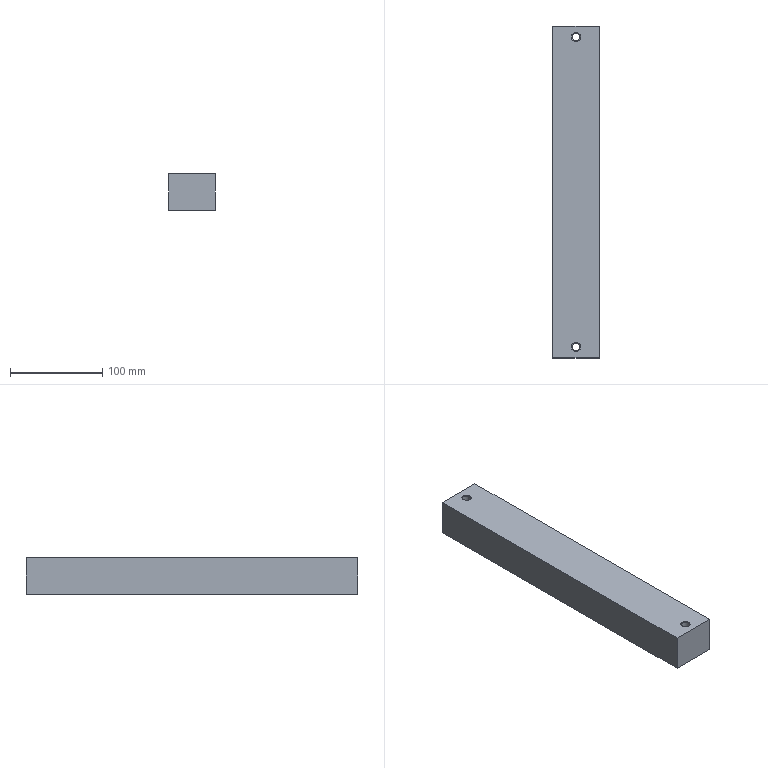Part | STEP file | 1 solid | 12 faces | box 50 x 360 x 40 mm | volume 715429 mm3 | plane 6 | cone 4 | cylinder 2 | commonest cylinder face diameters 8.5 x2
STEP:
#1=CARTESIAN_POINT('',(0.,0.,0.));
#2=DIRECTION('',(0.,0.,1.));
#3=DIRECTION('',(1.,0.,0.));
#4=AXIS2_PLACEMENT_3D('',#1,#2,#3);
#5=CARTESIAN_POINT('',(1866.247,274.48,93.619));
#6=VERTEX_POINT('',#5);
#7=CARTESIAN_POINT('',(1871.247,274.48,93.619));
#8=DIRECTION('',(0.,0.,1.));
#9=DIRECTION('',(-1.,0.,0.));
#10=AXIS2_PLACEMENT_3D('',#7,#8,#9);
#11=CIRCLE('',#10,5.);
#12=CARTESIAN_POINT('',(1846.247,622.48,93.619));
#13=DIRECTION('',(0.,0.,-1.));
#14=DIRECTION('',(0.,1.,0.));
#15=AXIS2_PLACEMENT_3D('',#12,#13,#14);
#16=PLANE('',#15);
#17=CARTESIAN_POINT('',(-348.,20.));
#18=CARTESIAN_POINT('',(-356.66,20.));
#19=CARTESIAN_POINT('',(-352.33,27.5));
#20=CARTESIAN_POINT('',(-348.,35.));
#21=CARTESIAN_POINT('',(-343.67,27.5));
#22=CARTESIAN_POINT('',(-339.34,20.));
#23=CARTESIAN_POINT('',(-348.,20.));
#24=(BOUNDED_CURVE()B_SPLINE_CURVE(2,(#17,#18,#19,#20,#21,#22,#23),.UNSPECIFIED.,.T.,.F.)B_SPLINE_CURVE_WITH_KNOTS((1,2,2,2,2,1),(-2.094,0.,2.094,4.189,6.283,8.378),.UNSPECIFIED.)CURVE()GEOMETRIC_REPRESENTATION_ITEM()RATIONAL_B_SPLINE_CURVE((1.,0.5,1.,0.5,1.,0.5,1.))REPRESENTATION_ITEM(''));
#25=(GEOMETRIC_REPRESENTATION_CONTEXT(2)PARAMETRIC_REPRESENTATION_CONTEXT()REPRESENTATION_CONTEXT('',''));
#26=DEFINITIONAL_REPRESENTATION('',(#24),#25);
#27=PCURVE('',#16,#26);
#28=CARTESIAN_POINT('',(1871.247,274.48,93.619));
#29=DIRECTION('',(0.,0.,-1.));
#30=DIRECTION('',(1.,0.,0.));
#31=AXIS2_PLACEMENT_3D('',#28,#29,#30);
#32=CONICAL_SURFACE('',#31,5.,0.7854);
#33=CARTESIAN_POINT('',(9.425,0.));
#34=DIRECTION('',(-1.,0.));
#35=VECTOR('',#34,1.);
#36=LINE('',#33,#35);
#37=(GEOMETRIC_REPRESENTATION_CONTEXT(2)PARAMETRIC_REPRESENTATION_CONTEXT()REPRESENTATION_CONTEXT('',''));
#38=DEFINITIONAL_REPRESENTATION('',(#36),#37);
#39=PCURVE('',#32,#38);
#40=SURFACE_CURVE('',#11,(#27,#39),.PCURVE_S1.);
#41=EDGE_CURVE('',#6,#6,#40,.T.);
#42=ORIENTED_EDGE('',*,*,#41,.T.);
#43=EDGE_LOOP('',(#42));
#44=FACE_BOUND('',#43,.T.);
#45=CARTESIAN_POINT('',(1866.247,610.48,93.619));
#46=VERTEX_POINT('',#45);
#47=CARTESIAN_POINT('',(1871.247,610.48,93.619));
#48=DIRECTION('',(0.,0.,1.));
#49=DIRECTION('',(-1.,0.,0.));
#50=AXIS2_PLACEMENT_3D('',#47,#48,#49);
#51=CIRCLE('',#50,5.);
#52=CARTESIAN_POINT('',(-12.,20.));
#53=CARTESIAN_POINT('',(-20.66,20.));
#54=CARTESIAN_POINT('',(-16.33,27.5));
#55=CARTESIAN_POINT('',(-12.,35.));
#56=CARTESIAN_POINT('',(-7.67,27.5));
#57=CARTESIAN_POINT('',(-3.34,20.));
#58=CARTESIAN_POINT('',(-12.,20.));
#59=(BOUNDED_CURVE()B_SPLINE_CURVE(2,(#52,#53,#54,#55,#56,#57,#58),.UNSPECIFIED.,.T.,.F.)B_SPLINE_CURVE_WITH_KNOTS((1,2,2,2,2,1),(-2.094,0.,2.094,4.189,6.283,8.378),.UNSPECIFIED.)CURVE()GEOMETRIC_REPRESENTATION_ITEM()RATIONAL_B_SPLINE_CURVE((1.,0.5,1.,0.5,1.,0.5,1.))REPRESENTATION_ITEM(''));
#60=(GEOMETRIC_REPRESENTATION_CONTEXT(2)PARAMETRIC_REPRESENTATION_CONTEXT()REPRESENTATION_CONTEXT('',''));
#61=DEFINITIONAL_REPRESENTATION('',(#59),#60);
#62=PCURVE('',#16,#61);
#63=CARTESIAN_POINT('',(1871.247,610.48,93.619));
#64=DIRECTION('',(0.,0.,-1.));
#65=DIRECTION('',(1.,0.,0.));
#66=AXIS2_PLACEMENT_3D('',#63,#64,#65);
#67=CONICAL_SURFACE('',#66,5.,0.7854);
#68=CARTESIAN_POINT('',(9.425,0.));
#69=DIRECTION('',(-1.,0.));
#70=VECTOR('',#69,1.);
#71=LINE('',#68,#70);
#72=(GEOMETRIC_REPRESENTATION_CONTEXT(2)PARAMETRIC_REPRESENTATION_CONTEXT()REPRESENTATION_CONTEXT('',''));
#73=DEFINITIONAL_REPRESENTATION('',(#71),#72);
#74=PCURVE('',#67,#73);
#75=SURFACE_CURVE('',#51,(#62,#74),.PCURVE_S1.);
#76=EDGE_CURVE('',#46,#46,#75,.T.);
#77=ORIENTED_EDGE('',*,*,#76,.T.);
#78=EDGE_LOOP('',(#77));
#79=FACE_BOUND('',#78,.T.);
#80=CARTESIAN_POINT('',(1846.247,262.48,93.619));
#81=VERTEX_POINT('',#80);
#82=CARTESIAN_POINT('',(1896.247,262.48,93.619));
#83=VERTEX_POINT('',#82);
#84=CARTESIAN_POINT('',(1846.247,262.48,93.619));
#85=DIRECTION('',(1.,0.,0.));
#86=VECTOR('',#85,1.);
#87=LINE('',#84,#86);
#88=CARTESIAN_POINT('',(-360.,0.));
#89=DIRECTION('',(0.,1.));
#90=VECTOR('',#89,1.);
#91=LINE('',#88,#90);
#92=(GEOMETRIC_REPRESENTATION_CONTEXT(2)PARAMETRIC_REPRESENTATION_CONTEXT()REPRESENTATION_CONTEXT('',''));
#93=DEFINITIONAL_REPRESENTATION('',(#91),#92);
#94=PCURVE('',#16,#93);
#95=CARTESIAN_POINT('',(1846.247,262.48,93.619));
#96=DIRECTION('',(0.,-1.,0.));
#97=DIRECTION('',(0.,0.,-1.));
#98=AXIS2_PLACEMENT_3D('',#95,#96,#97);
#99=PLANE('',#98);
#100=CARTESIAN_POINT('',(0.,0.));
#101=DIRECTION('',(0.,1.));
#102=VECTOR('',#101,1.);
#103=LINE('',#100,#102);
#104=(GEOMETRIC_REPRESENTATION_CONTEXT(2)PARAMETRIC_REPRESENTATION_CONTEXT()REPRESENTATION_CONTEXT('',''));
#105=DEFINITIONAL_REPRESENTATION('',(#103),#104);
#106=PCURVE('',#99,#105);
#107=SURFACE_CURVE('',#87,(#94,#106),.PCURVE_S1.);
#108=EDGE_CURVE('',#81,#83,#107,.T.);
#109=ORIENTED_EDGE('',*,*,#108,.F.);
#110=CARTESIAN_POINT('',(1846.247,622.48,93.619));
#111=VERTEX_POINT('',#110);
#112=CARTESIAN_POINT('',(1846.247,622.48,93.619));
#113=DIRECTION('',(0.,-1.,0.));
#114=VECTOR('',#113,1.);
#115=LINE('',#112,#114);
#116=CARTESIAN_POINT('',(0.,0.));
#117=DIRECTION('',(-1.,0.));
#118=VECTOR('',#117,1.);
#119=LINE('',#116,#118);
#120=(GEOMETRIC_REPRESENTATION_CONTEXT(2)PARAMETRIC_REPRESENTATION_CONTEXT()REPRESENTATION_CONTEXT('',''));
#121=DEFINITIONAL_REPRESENTATION('',(#119),#120);
#122=PCURVE('',#16,#121);
#123=CARTESIAN_POINT('',(1846.247,622.48,93.619));
#124=DIRECTION('',(-1.,0.,0.));
#125=DIRECTION('',(0.,1.,0.));
#126=AXIS2_PLACEMENT_3D('',#123,#124,#125);
#127=PLANE('',#126);
#128=CARTESIAN_POINT('',(0.,0.));
#129=DIRECTION('',(-1.,0.));
#130=VECTOR('',#129,1.);
#131=LINE('',#128,#130);
#132=(GEOMETRIC_REPRESENTATION_CONTEXT(2)PARAMETRIC_REPRESENTATION_CONTEXT()REPRESENTATION_CONTEXT('',''));
#133=DEFINITIONAL_REPRESENTATION('',(#131),#132);
#134=PCURVE('',#127,#133);
#135=SURFACE_CURVE('',#115,(#122,#134),.PCURVE_S1.);
#136=EDGE_CURVE('',#111,#81,#135,.T.);
#137=ORIENTED_EDGE('',*,*,#136,.F.);
#138=CARTESIAN_POINT('',(1896.247,622.48,93.619));
#139=VERTEX_POINT('',#138);
#140=CARTESIAN_POINT('',(1846.247,622.48,93.619));
#141=DIRECTION('',(1.,0.,0.));
#142=VECTOR('',#141,1.);
#143=LINE('',#140,#142);
#144=CARTESIAN_POINT('',(0.,0.));
#145=DIRECTION('',(0.,1.));
#146=VECTOR('',#145,1.);
#147=LINE('',#144,#146);
#148=(GEOMETRIC_REPRESENTATION_CONTEXT(2)PARAMETRIC_REPRESENTATION_CONTEXT()REPRESENTATION_CONTEXT('',''));
#149=DEFINITIONAL_REPRESENTATION('',(#147),#148);
#150=PCURVE('',#16,#149);
#151=CARTESIAN_POINT('',(1846.247,622.48,93.619));
#152=DIRECTION('',(0.,-1.,0.));
#153=DIRECTION('',(0.,0.,-1.));
#154=AXIS2_PLACEMENT_3D('',#151,#152,#153);
#155=PLANE('',#154);
#156=CARTESIAN_POINT('',(0.,0.));
#157=DIRECTION('',(0.,1.));
#158=VECTOR('',#157,1.);
#159=LINE('',#156,#158);
#160=(GEOMETRIC_REPRESENTATION_CONTEXT(2)PARAMETRIC_REPRESENTATION_CONTEXT()REPRESENTATION_CONTEXT('',''));
#161=DEFINITIONAL_REPRESENTATION('',(#159),#160);
#162=PCURVE('',#155,#161);
#163=SURFACE_CURVE('',#143,(#150,#162),.PCURVE_S1.);
#164=EDGE_CURVE('',#111,#139,#163,.T.);
#165=ORIENTED_EDGE('',*,*,#164,.T.);
#166=CARTESIAN_POINT('',(1896.247,622.48,93.619));
#167=DIRECTION('',(0.,-1.,0.));
#168=VECTOR('',#167,1.);
#169=LINE('',#166,#168);
#170=CARTESIAN_POINT('',(0.,50.));
#171=DIRECTION('',(-1.,0.));
#172=VECTOR('',#171,1.);
#173=LINE('',#170,#172);
#174=(GEOMETRIC_REPRESENTATION_CONTEXT(2)PARAMETRIC_REPRESENTATION_CONTEXT()REPRESENTATION_CONTEXT('',''));
#175=DEFINITIONAL_REPRESENTATION('',(#173),#174);
#176=PCURVE('',#16,#175);
#177=CARTESIAN_POINT('',(1896.247,622.48,93.619));
#178=DIRECTION('',(-1.,0.,0.));
#179=DIRECTION('',(0.,1.,0.));
#180=AXIS2_PLACEMENT_3D('',#177,#178,#179);
#181=PLANE('',#180);
#182=CARTESIAN_POINT('',(0.,0.));
#183=DIRECTION('',(-1.,0.));
#184=VECTOR('',#183,1.);
#185=LINE('',#182,#184);
#186=(GEOMETRIC_REPRESENTATION_CONTEXT(2)PARAMETRIC_REPRESENTATION_CONTEXT()REPRESENTATION_CONTEXT('',''));
#187=DEFINITIONAL_REPRESENTATION('',(#185),#186);
#188=PCURVE('',#181,#187);
#189=SURFACE_CURVE('',#169,(#176,#188),.PCURVE_S1.);
#190=EDGE_CURVE('',#139,#83,#189,.T.);
#191=ORIENTED_EDGE('',*,*,#190,.T.);
#192=EDGE_LOOP('',(#109,#137,#165,#191));
#193=FACE_BOUND('',#192,.T.);
#194=ADVANCED_FACE('',(#44,#79,#193),#16,.T.);
#195=ORIENTED_EDGE('',*,*,#164,.F.);
#196=CARTESIAN_POINT('',(1846.247,622.48,133.619));
#197=VERTEX_POINT('',#196);
#198=CARTESIAN_POINT('',(1846.247,622.48,93.619));
#199=DIRECTION('',(0.,0.,-1.));
#200=VECTOR('',#199,1.);
#201=LINE('',#198,#200);
#202=CARTESIAN_POINT('',(0.,0.));
#203=DIRECTION('',(1.,0.));
#204=VECTOR('',#203,1.);
#205=LINE('',#202,#204);
#206=(GEOMETRIC_REPRESENTATION_CONTEXT(2)PARAMETRIC_REPRESENTATION_CONTEXT()REPRESENTATION_CONTEXT('',''));
#207=DEFINITIONAL_REPRESENTATION('',(#205),#206);
#208=PCURVE('',#155,#207);
#209=CARTESIAN_POINT('',(0.,0.));
#210=DIRECTION('',(0.,1.));
#211=VECTOR('',#210,1.);
#212=LINE('',#209,#211);
#213=(GEOMETRIC_REPRESENTATION_CONTEXT(2)PARAMETRIC_REPRESENTATION_CONTEXT()REPRESENTATION_CONTEXT('',''));
#214=DEFINITIONAL_REPRESENTATION('',(#212),#213);
#215=PCURVE('',#127,#214);
#216=SURFACE_CURVE('',#201,(#208,#215),.PCURVE_S1.);
#217=EDGE_CURVE('',#197,#111,#216,.T.);
#218=ORIENTED_EDGE('',*,*,#217,.F.);
#219=CARTESIAN_POINT('',(1896.247,622.48,133.619));
#220=VERTEX_POINT('',#219);
#221=CARTESIAN_POINT('',(1846.247,622.48,133.619));
#222=DIRECTION('',(1.,0.,0.));
#223=VECTOR('',#222,1.);
#224=LINE('',#221,#223);
#225=CARTESIAN_POINT('',(-40.,0.));
#226=DIRECTION('',(0.,1.));
#227=VECTOR('',#226,1.);
#228=LINE('',#225,#227);
#229=(GEOMETRIC_REPRESENTATION_CONTEXT(2)PARAMETRIC_REPRESENTATION_CONTEXT()REPRESENTATION_CONTEXT('',''));
#230=DEFINITIONAL_REPRESENTATION('',(#228),#229);
#231=PCURVE('',#155,#230);
#232=CARTESIAN_POINT('',(1846.247,622.48,133.619));
#233=DIRECTION('',(0.,0.,-1.));
#234=DIRECTION('',(0.,1.,0.));
#235=AXIS2_PLACEMENT_3D('',#232,#233,#234);
#236=PLANE('',#235);
#237=CARTESIAN_POINT('',(0.,0.));
#238=DIRECTION('',(0.,1.));
#239=VECTOR('',#238,1.);
#240=LINE('',#237,#239);
#241=(GEOMETRIC_REPRESENTATION_CONTEXT(2)PARAMETRIC_REPRESENTATION_CONTEXT()REPRESENTATION_CONTEXT('',''));
#242=DEFINITIONAL_REPRESENTATION('',(#240),#241);
#243=PCURVE('',#236,#242);
#244=SURFACE_CURVE('',#224,(#231,#243),.PCURVE_S1.);
#245=EDGE_CURVE('',#197,#220,#244,.T.);
#246=ORIENTED_EDGE('',*,*,#245,.T.);
#247=CARTESIAN_POINT('',(1896.247,622.48,93.619));
#248=DIRECTION('',(0.,0.,-1.));
#249=VECTOR('',#248,1.);
#250=LINE('',#247,#249);
#251=CARTESIAN_POINT('',(0.,50.));
#252=DIRECTION('',(1.,0.));
#253=VECTOR('',#252,1.);
#254=LINE('',#251,#253);
#255=(GEOMETRIC_REPRESENTATION_CONTEXT(2)PARAMETRIC_REPRESENTATION_CONTEXT()REPRESENTATION_CONTEXT('',''));
#256=DEFINITIONAL_REPRESENTATION('',(#254),#255);
#257=PCURVE('',#155,#256);
#258=CARTESIAN_POINT('',(0.,0.));
#259=DIRECTION('',(0.,1.));
#260=VECTOR('',#259,1.);
#261=LINE('',#258,#260);
#262=(GEOMETRIC_REPRESENTATION_CONTEXT(2)PARAMETRIC_REPRESENTATION_CONTEXT()REPRESENTATION_CONTEXT('',''));
#263=DEFINITIONAL_REPRESENTATION('',(#261),#262);
#264=PCURVE('',#181,#263);
#265=SURFACE_CURVE('',#250,(#257,#264),.PCURVE_S1.);
#266=EDGE_CURVE('',#220,#139,#265,.T.);
#267=ORIENTED_EDGE('',*,*,#266,.T.);
#268=EDGE_LOOP('',(#195,#218,#246,#267));
#269=FACE_BOUND('',#268,.T.);
#270=ADVANCED_FACE('',(#269),#155,.F.);
#271=CARTESIAN_POINT('',(1866.247,274.48,133.619));
#272=VERTEX_POINT('',#271);
#273=CARTESIAN_POINT('',(1871.247,274.48,133.619));
#274=DIRECTION('',(0.,0.,-1.));
#275=DIRECTION('',(-1.,0.,0.));
#276=AXIS2_PLACEMENT_3D('',#273,#274,#275);
#277=CIRCLE('',#276,5.);
#278=CARTESIAN_POINT('',(-348.,25.));
#279=DIRECTION('',(0.,-1.));
#280=AXIS2_PLACEMENT_2D('',#278,#279);
#281=CIRCLE('',#280,5.);
#282=(GEOMETRIC_REPRESENTATION_CONTEXT(2)PARAMETRIC_REPRESENTATION_CONTEXT()REPRESENTATION_CONTEXT('',''));
#283=DEFINITIONAL_REPRESENTATION('',(#281),#282);
#284=PCURVE('',#236,#283);
#285=CARTESIAN_POINT('',(1871.247,274.48,132.869));
#286=DIRECTION('',(0.,0.,1.));
#287=DIRECTION('',(-1.,0.,0.));
#288=AXIS2_PLACEMENT_3D('',#285,#286,#287);
#289=CONICAL_SURFACE('',#288,4.25,0.7854);
#290=CARTESIAN_POINT('',(6.283,0.75));
#291=DIRECTION('',(-1.,0.));
#292=VECTOR('',#291,1.);
#293=LINE('',#290,#292);
#294=(GEOMETRIC_REPRESENTATION_CONTEXT(2)PARAMETRIC_REPRESENTATION_CONTEXT()REPRESENTATION_CONTEXT('',''));
#295=DEFINITIONAL_REPRESENTATION('',(#293),#294);
#296=PCURVE('',#289,#295);
#297=SURFACE_CURVE('',#277,(#284,#296),.PCURVE_S1.);
#298=EDGE_CURVE('',#272,#272,#297,.T.);
#299=ORIENTED_EDGE('',*,*,#298,.T.);
#300=EDGE_LOOP('',(#299));
#301=FACE_BOUND('',#300,.T.);
#302=CARTESIAN_POINT('',(1866.247,610.48,133.619));
#303=VERTEX_POINT('',#302);
#304=CARTESIAN_POINT('',(1871.247,610.48,133.619));
#305=DIRECTION('',(0.,0.,-1.));
#306=DIRECTION('',(-1.,0.,0.));
#307=AXIS2_PLACEMENT_3D('',#304,#305,#306);
#308=CIRCLE('',#307,5.);
#309=CARTESIAN_POINT('',(-12.,25.));
#310=DIRECTION('',(0.,-1.));
#311=AXIS2_PLACEMENT_2D('',#309,#310);
#312=CIRCLE('',#311,5.);
#313=(GEOMETRIC_REPRESENTATION_CONTEXT(2)PARAMETRIC_REPRESENTATION_CONTEXT()REPRESENTATION_CONTEXT('',''));
#314=DEFINITIONAL_REPRESENTATION('',(#312),#313);
#315=PCURVE('',#236,#314);
#316=CARTESIAN_POINT('',(1871.247,610.48,132.869));
#317=DIRECTION('',(0.,0.,1.));
#318=DIRECTION('',(-1.,0.,0.));
#319=AXIS2_PLACEMENT_3D('',#316,#317,#318);
#320=CONICAL_SURFACE('',#319,4.25,0.7854);
#321=CARTESIAN_POINT('',(6.283,0.75));
#322=DIRECTION('',(-1.,0.));
#323=VECTOR('',#322,1.);
#324=LINE('',#321,#323);
#325=(GEOMETRIC_REPRESENTATION_CONTEXT(2)PARAMETRIC_REPRESENTATION_CONTEXT()REPRESENTATION_CONTEXT('',''));
#326=DEFINITIONAL_REPRESENTATION('',(#324),#325);
#327=PCURVE('',#320,#326);
#328=SURFACE_CURVE('',#308,(#315,#327),.PCURVE_S1.);
#329=EDGE_CURVE('',#303,#303,#328,.T.);
#330=ORIENTED_EDGE('',*,*,#329,.T.);
#331=EDGE_LOOP('',(#330));
#332=FACE_BOUND('',#331,.T.);
#333=ORIENTED_EDGE('',*,*,#245,.F.);
#334=CARTESIAN_POINT('',(1846.247,262.48,133.619));
#335=VERTEX_POINT('',#334);
#336=CARTESIAN_POINT('',(1846.247,622.48,133.619));
#337=DIRECTION('',(0.,1.,0.));
#338=VECTOR('',#337,1.);
#339=LINE('',#336,#338);
#340=CARTESIAN_POINT('',(0.,0.));
#341=DIRECTION('',(1.,0.));
#342=VECTOR('',#341,1.);
#343=LINE('',#340,#342);
#344=(GEOMETRIC_REPRESENTATION_CONTEXT(2)PARAMETRIC_REPRESENTATION_CONTEXT()REPRESENTATION_CONTEXT('',''));
#345=DEFINITIONAL_REPRESENTATION('',(#343),#344);
#346=PCURVE('',#236,#345);
#347=CARTESIAN_POINT('',(0.,-40.));
#348=DIRECTION('',(1.,0.));
#349=VECTOR('',#348,1.);
#350=LINE('',#347,#349);
#351=(GEOMETRIC_REPRESENTATION_CONTEXT(2)PARAMETRIC_REPRESENTATION_CONTEXT()REPRESENTATION_CONTEXT('',''));
#352=DEFINITIONAL_REPRESENTATION('',(#350),#351);
#353=PCURVE('',#127,#352);
#354=SURFACE_CURVE('',#339,(#346,#353),.PCURVE_S1.);
#355=EDGE_CURVE('',#335,#197,#354,.T.);
#356=ORIENTED_EDGE('',*,*,#355,.F.);
#357=CARTESIAN_POINT('',(1896.247,262.48,133.619));
#358=VERTEX_POINT('',#357);
#359=CARTESIAN_POINT('',(1846.247,262.48,133.619));
#360=DIRECTION('',(1.,0.,0.));
#361=VECTOR('',#360,1.);
#362=LINE('',#359,#361);
#363=CARTESIAN_POINT('',(-360.,0.));
#364=DIRECTION('',(0.,1.));
#365=VECTOR('',#364,1.);
#366=LINE('',#363,#365);
#367=(GEOMETRIC_REPRESENTATION_CONTEXT(2)PARAMETRIC_REPRESENTATION_CONTEXT()REPRESENTATION_CONTEXT('',''));
#368=DEFINITIONAL_REPRESENTATION('',(#366),#367);
#369=PCURVE('',#236,#368);
#370=CARTESIAN_POINT('',(-40.,0.));
#371=DIRECTION('',(0.,1.));
#372=VECTOR('',#371,1.);
#373=LINE('',#370,#372);
#374=(GEOMETRIC_REPRESENTATION_CONTEXT(2)PARAMETRIC_REPRESENTATION_CONTEXT()REPRESENTATION_CONTEXT('',''));
#375=DEFINITIONAL_REPRESENTATION('',(#373),#374);
#376=PCURVE('',#99,#375);
#377=SURFACE_CURVE('',#362,(#369,#376),.PCURVE_S1.);
#378=EDGE_CURVE('',#335,#358,#377,.T.);
#379=ORIENTED_EDGE('',*,*,#378,.T.);
#380=CARTESIAN_POINT('',(1896.247,622.48,133.619));
#381=DIRECTION('',(0.,1.,0.));
#382=VECTOR('',#381,1.);
#383=LINE('',#380,#382);
#384=CARTESIAN_POINT('',(0.,50.));
#385=DIRECTION('',(1.,0.));
#386=VECTOR('',#385,1.);
#387=LINE('',#384,#386);
#388=(GEOMETRIC_REPRESENTATION_CONTEXT(2)PARAMETRIC_REPRESENTATION_CONTEXT()REPRESENTATION_CONTEXT('',''));
#389=DEFINITIONAL_REPRESENTATION('',(#387),#388);
#390=PCURVE('',#236,#389);
#391=CARTESIAN_POINT('',(0.,-40.));
#392=DIRECTION('',(1.,0.));
#393=VECTOR('',#392,1.);
#394=LINE('',#391,#393);
#395=(GEOMETRIC_REPRESENTATION_CONTEXT(2)PARAMETRIC_REPRESENTATION_CONTEXT()REPRESENTATION_CONTEXT('',''));
#396=DEFINITIONAL_REPRESENTATION('',(#394),#395);
#397=PCURVE('',#181,#396);
#398=SURFACE_CURVE('',#383,(#390,#397),.PCURVE_S1.);
#399=EDGE_CURVE('',#358,#220,#398,.T.);
#400=ORIENTED_EDGE('',*,*,#399,.T.);
#401=EDGE_LOOP('',(#333,#356,#379,#400));
#402=FACE_BOUND('',#401,.T.);
#403=ADVANCED_FACE('',(#301,#332,#402),#236,.F.);
#404=CARTESIAN_POINT('',(1846.247,262.48,93.619));
#405=DIRECTION('',(0.,0.,1.));
#406=VECTOR('',#405,1.);
#407=LINE('',#404,#406);
#408=CARTESIAN_POINT('',(0.,0.));
#409=DIRECTION('',(-1.,0.));
#410=VECTOR('',#409,1.);
#411=LINE('',#408,#410);
#412=(GEOMETRIC_REPRESENTATION_CONTEXT(2)PARAMETRIC_REPRESENTATION_CONTEXT()REPRESENTATION_CONTEXT('',''));
#413=DEFINITIONAL_REPRESENTATION('',(#411),#412);
#414=PCURVE('',#99,#413);
#415=CARTESIAN_POINT('',(-360.,0.));
#416=DIRECTION('',(0.,-1.));
#417=VECTOR('',#416,1.);
#418=LINE('',#415,#417);
#419=(GEOMETRIC_REPRESENTATION_CONTEXT(2)PARAMETRIC_REPRESENTATION_CONTEXT()REPRESENTATION_CONTEXT('',''));
#420=DEFINITIONAL_REPRESENTATION('',(#418),#419);
#421=PCURVE('',#127,#420);
#422=SURFACE_CURVE('',#407,(#414,#421),.PCURVE_S1.);
#423=EDGE_CURVE('',#81,#335,#422,.T.);
#424=ORIENTED_EDGE('',*,*,#423,.F.);
#425=ORIENTED_EDGE('',*,*,#108,.T.);
#426=CARTESIAN_POINT('',(1896.247,262.48,93.619));
#427=DIRECTION('',(0.,0.,1.));
#428=VECTOR('',#427,1.);
#429=LINE('',#426,#428);
#430=CARTESIAN_POINT('',(0.,50.));
#431=DIRECTION('',(-1.,0.));
#432=VECTOR('',#431,1.);
#433=LINE('',#430,#432);
#434=(GEOMETRIC_REPRESENTATION_CONTEXT(2)PARAMETRIC_REPRESENTATION_CONTEXT()REPRESENTATION_CONTEXT('',''));
#435=DEFINITIONAL_REPRESENTATION('',(#433),#434);
#436=PCURVE('',#99,#435);
#437=CARTESIAN_POINT('',(-360.,0.));
#438=DIRECTION('',(0.,-1.));
#439=VECTOR('',#438,1.);
#440=LINE('',#437,#439);
#441=(GEOMETRIC_REPRESENTATION_CONTEXT(2)PARAMETRIC_REPRESENTATION_CONTEXT()REPRESENTATION_CONTEXT('',''));
#442=DEFINITIONAL_REPRESENTATION('',(#440),#441);
#443=PCURVE('',#181,#442);
#444=SURFACE_CURVE('',#429,(#436,#443),.PCURVE_S1.);
#445=EDGE_CURVE('',#83,#358,#444,.T.);
#446=ORIENTED_EDGE('',*,*,#445,.T.);
#447=ORIENTED_EDGE('',*,*,#378,.F.);
#448=EDGE_LOOP('',(#424,#425,#446,#447));
#449=FACE_BOUND('',#448,.T.);
#450=ADVANCED_FACE('',(#449),#99,.T.);
#451=ORIENTED_EDGE('',*,*,#399,.F.);
#452=ORIENTED_EDGE('',*,*,#445,.F.);
#453=ORIENTED_EDGE('',*,*,#190,.F.);
#454=ORIENTED_EDGE('',*,*,#266,.F.);
#455=EDGE_LOOP('',(#451,#452,#453,#454));
#456=FACE_BOUND('',#455,.T.);
#457=ADVANCED_FACE('',(#456),#181,.F.);
#458=ORIENTED_EDGE('',*,*,#355,.T.);
#459=ORIENTED_EDGE('',*,*,#217,.T.);
#460=ORIENTED_EDGE('',*,*,#136,.T.);
#461=ORIENTED_EDGE('',*,*,#423,.T.);
#462=EDGE_LOOP('',(#458,#459,#460,#461));
#463=FACE_BOUND('',#462,.T.);
#464=ADVANCED_FACE('',(#463),#127,.T.);
#465=CARTESIAN_POINT('',(1866.997,610.48,132.869));
#466=VERTEX_POINT('',#465);
#467=CARTESIAN_POINT('',(1875.497,610.48,132.869));
#468=VERTEX_POINT('',#467);
#469=CARTESIAN_POINT('',(1871.247,610.48,132.869));
#470=DIRECTION('',(0.,0.,1.));
#471=DIRECTION('',(1.,0.,0.));
#472=AXIS2_PLACEMENT_3D('',#469,#470,#471);
#473=CIRCLE('',#472,4.25);
#474=CARTESIAN_POINT('',(1871.247,610.48,93.619));
#475=DIRECTION('',(0.,0.,1.));
#476=DIRECTION('',(-1.,0.,0.));
#477=AXIS2_PLACEMENT_3D('',#474,#475,#476);
#478=CYLINDRICAL_SURFACE('',#477,4.25);
#479=CARTESIAN_POINT('',(-3.142,39.25));
#480=DIRECTION('',(1.,0.));
#481=VECTOR('',#480,1.);
#482=LINE('',#479,#481);
#483=(GEOMETRIC_REPRESENTATION_CONTEXT(2)PARAMETRIC_REPRESENTATION_CONTEXT()REPRESENTATION_CONTEXT('',''));
#484=DEFINITIONAL_REPRESENTATION('',(#482),#483);
#485=PCURVE('',#478,#484);
#486=CARTESIAN_POINT('',(-3.142,0.));
#487=DIRECTION('',(1.,0.));
#488=VECTOR('',#487,1.);
#489=LINE('',#486,#488);
#490=(GEOMETRIC_REPRESENTATION_CONTEXT(2)PARAMETRIC_REPRESENTATION_CONTEXT()REPRESENTATION_CONTEXT('',''));
#491=DEFINITIONAL_REPRESENTATION('',(#489),#490);
#492=PCURVE('',#320,#491);
#493=SURFACE_CURVE('',#473,(#485,#492),.PCURVE_S1.);
#494=EDGE_CURVE('',#466,#468,#493,.T.);
#495=ORIENTED_EDGE('',*,*,#494,.F.);
#496=CARTESIAN_POINT('',(1866.997,610.48,94.369));
#497=VERTEX_POINT('',#496);
#498=CARTESIAN_POINT('',(1866.997,610.48,94.369));
#499=CARTESIAN_POINT('',(1866.997,610.48,132.869));
#500=B_SPLINE_CURVE_WITH_KNOTS('',1,(#498,#499),.UNSPECIFIED.,.F.,.F.,(2,2),(0.75,39.25),.PIECEWISE_BEZIER_KNOTS.);
#501=CARTESIAN_POINT('',(0.,0.));
#502=DIRECTION('',(0.,1.));
#503=VECTOR('',#502,1.);
#504=LINE('',#501,#503);
#505=(GEOMETRIC_REPRESENTATION_CONTEXT(2)PARAMETRIC_REPRESENTATION_CONTEXT()REPRESENTATION_CONTEXT('',''));
#506=DEFINITIONAL_REPRESENTATION('',(#504),#505);
#507=PCURVE('',#478,#506);
#508=CARTESIAN_POINT('',(6.283,0.));
#509=DIRECTION('',(0.,1.));
#510=VECTOR('',#509,1.);
#511=LINE('',#508,#510);
#512=(GEOMETRIC_REPRESENTATION_CONTEXT(2)PARAMETRIC_REPRESENTATION_CONTEXT()REPRESENTATION_CONTEXT('',''));
#513=DEFINITIONAL_REPRESENTATION('',(#511),#512);
#514=PCURVE('',#478,#513);
#515=SEAM_CURVE('',#500,(#507,#514),.PCURVE_S1.);
#516=EDGE_CURVE('',#497,#466,#515,.T.);
#517=ORIENTED_EDGE('',*,*,#516,.F.);
#518=CARTESIAN_POINT('',(1871.247,610.48,94.369));
#519=DIRECTION('',(0.,0.,-1.));
#520=DIRECTION('',(-1.,0.,0.));
#521=AXIS2_PLACEMENT_3D('',#518,#519,#520);
#522=CIRCLE('',#521,4.25);
#523=CARTESIAN_POINT('',(6.283,0.75));
#524=DIRECTION('',(-1.,0.));
#525=VECTOR('',#524,1.);
#526=LINE('',#523,#525);
#527=(GEOMETRIC_REPRESENTATION_CONTEXT(2)PARAMETRIC_REPRESENTATION_CONTEXT()REPRESENTATION_CONTEXT('',''));
#528=DEFINITIONAL_REPRESENTATION('',(#526),#527);
#529=PCURVE('',#478,#528);
#530=CARTESIAN_POINT('',(3.142,-0.75));
#531=DIRECTION('',(1.,0.));
#532=VECTOR('',#531,1.);
#533=LINE('',#530,#532);
#534=(GEOMETRIC_REPRESENTATION_CONTEXT(2)PARAMETRIC_REPRESENTATION_CONTEXT()REPRESENTATION_CONTEXT('',''));
#535=DEFINITIONAL_REPRESENTATION('',(#533),#534);
#536=PCURVE('',#67,#535);
#537=SURFACE_CURVE('',#522,(#529,#536),.PCURVE_S1.);
#538=EDGE_CURVE('',#497,#497,#537,.T.);
#539=ORIENTED_EDGE('',*,*,#538,.F.);
#540=ORIENTED_EDGE('',*,*,#516,.T.);
#541=CARTESIAN_POINT('',(1871.247,610.48,132.869));
#542=DIRECTION('',(0.,0.,1.));
#543=DIRECTION('',(1.,0.,0.));
#544=AXIS2_PLACEMENT_3D('',#541,#542,#543);
#545=CIRCLE('',#544,4.25);
#546=CARTESIAN_POINT('',(3.142,39.25));
#547=DIRECTION('',(1.,0.));
#548=VECTOR('',#547,1.);
#549=LINE('',#546,#548);
#550=(GEOMETRIC_REPRESENTATION_CONTEXT(2)PARAMETRIC_REPRESENTATION_CONTEXT()REPRESENTATION_CONTEXT('',''));
#551=DEFINITIONAL_REPRESENTATION('',(#549),#550);
#552=PCURVE('',#478,#551);
#553=CARTESIAN_POINT('',(3.142,0.));
#554=DIRECTION('',(1.,0.));
#555=VECTOR('',#554,1.);
#556=LINE('',#553,#555);
#557=(GEOMETRIC_REPRESENTATION_CONTEXT(2)PARAMETRIC_REPRESENTATION_CONTEXT()REPRESENTATION_CONTEXT('',''));
#558=DEFINITIONAL_REPRESENTATION('',(#556),#557);
#559=PCURVE('',#320,#558);
#560=SURFACE_CURVE('',#545,(#552,#559),.PCURVE_S1.);
#561=EDGE_CURVE('',#468,#466,#560,.T.);
#562=ORIENTED_EDGE('',*,*,#561,.F.);
#563=EDGE_LOOP('',(#495,#517,#539,#540,#562));
#564=FACE_BOUND('',#563,.F.);
#565=ADVANCED_FACE('',(#564),#478,.F.);
#566=ORIENTED_EDGE('',*,*,#538,.T.);
#567=CARTESIAN_POINT('',(1866.997,610.48,94.369));
#568=CARTESIAN_POINT('',(1866.247,610.48,93.619));
#569=B_SPLINE_CURVE_WITH_KNOTS('',1,(#567,#568),.UNSPECIFIED.,.F.,.F.,(2,2),(-1.061,0.),.PIECEWISE_BEZIER_KNOTS.);
#570=CARTESIAN_POINT('',(9.425,0.));
#571=DIRECTION('',(0.,1.));
#572=VECTOR('',#571,1.);
#573=LINE('',#570,#572);
#574=(GEOMETRIC_REPRESENTATION_CONTEXT(2)PARAMETRIC_REPRESENTATION_CONTEXT()REPRESENTATION_CONTEXT('',''));
#575=DEFINITIONAL_REPRESENTATION('',(#573),#574);
#576=PCURVE('',#67,#575);
#577=CARTESIAN_POINT('',(3.142,0.));
#578=DIRECTION('',(0.,1.));
#579=VECTOR('',#578,1.);
#580=LINE('',#577,#579);
#581=(GEOMETRIC_REPRESENTATION_CONTEXT(2)PARAMETRIC_REPRESENTATION_CONTEXT()REPRESENTATION_CONTEXT('',''));
#582=DEFINITIONAL_REPRESENTATION('',(#580),#581);
#583=PCURVE('',#67,#582);
#584=SEAM_CURVE('',#569,(#576,#583),.PCURVE_S1.);
#585=EDGE_CURVE('',#497,#46,#584,.T.);
#586=ORIENTED_EDGE('',*,*,#585,.T.);
#587=ORIENTED_EDGE('',*,*,#76,.T.);
#588=ORIENTED_EDGE('',*,*,#585,.F.);
#589=EDGE_LOOP('',(#566,#586,#587,#588));
#590=FACE_BOUND('',#589,.F.);
#591=ADVANCED_FACE('',(#590),#67,.F.);
#592=ORIENTED_EDGE('',*,*,#329,.T.);
#593=CARTESIAN_POINT('',(1866.997,610.48,132.869));
#594=CARTESIAN_POINT('',(1866.247,610.48,133.619));
#595=B_SPLINE_CURVE_WITH_KNOTS('',1,(#593,#594),.UNSPECIFIED.,.F.,.F.,(2,2),(0.,1.061),.PIECEWISE_BEZIER_KNOTS.);
#596=CARTESIAN_POINT('',(0.,0.));
#597=DIRECTION('',(0.,1.));
#598=VECTOR('',#597,1.);
#599=LINE('',#596,#598);
#600=(GEOMETRIC_REPRESENTATION_CONTEXT(2)PARAMETRIC_REPRESENTATION_CONTEXT()REPRESENTATION_CONTEXT('',''));
#601=DEFINITIONAL_REPRESENTATION('',(#599),#600);
#602=PCURVE('',#320,#601);
#603=CARTESIAN_POINT('',(6.283,0.));
#604=DIRECTION('',(0.,1.));
#605=VECTOR('',#604,1.);
#606=LINE('',#603,#605);
#607=(GEOMETRIC_REPRESENTATION_CONTEXT(2)PARAMETRIC_REPRESENTATION_CONTEXT()REPRESENTATION_CONTEXT('',''));
#608=DEFINITIONAL_REPRESENTATION('',(#606),#607);
#609=PCURVE('',#320,#608);
#610=SEAM_CURVE('',#595,(#602,#609),.PCURVE_S1.);
#611=EDGE_CURVE('',#466,#303,#610,.T.);
#612=ORIENTED_EDGE('',*,*,#611,.F.);
#613=ORIENTED_EDGE('',*,*,#494,.T.);
#614=ORIENTED_EDGE('',*,*,#561,.T.);
#615=ORIENTED_EDGE('',*,*,#611,.T.);
#616=EDGE_LOOP('',(#592,#612,#613,#614,#615));
#617=FACE_BOUND('',#616,.F.);
#618=ADVANCED_FACE('',(#617),#320,.F.);
#619=CARTESIAN_POINT('',(1866.997,274.48,132.869));
#620=VERTEX_POINT('',#619);
#621=CARTESIAN_POINT('',(1875.497,274.48,132.869));
#622=VERTEX_POINT('',#621);
#623=CARTESIAN_POINT('',(1871.247,274.48,132.869));
#624=DIRECTION('',(0.,0.,1.));
#625=DIRECTION('',(1.,0.,0.));
#626=AXIS2_PLACEMENT_3D('',#623,#624,#625);
#627=CIRCLE('',#626,4.25);
#628=CARTESIAN_POINT('',(1871.247,274.48,93.619));
#629=DIRECTION('',(0.,0.,1.));
#630=DIRECTION('',(-1.,0.,0.));
#631=AXIS2_PLACEMENT_3D('',#628,#629,#630);
#632=CYLINDRICAL_SURFACE('',#631,4.25);
#633=CARTESIAN_POINT('',(-3.142,39.25));
#634=DIRECTION('',(1.,0.));
#635=VECTOR('',#634,1.);
#636=LINE('',#633,#635);
#637=(GEOMETRIC_REPRESENTATION_CONTEXT(2)PARAMETRIC_REPRESENTATION_CONTEXT()REPRESENTATION_CONTEXT('',''));
#638=DEFINITIONAL_REPRESENTATION('',(#636),#637);
#639=PCURVE('',#632,#638);
#640=CARTESIAN_POINT('',(-3.142,0.));
#641=DIRECTION('',(1.,0.));
#642=VECTOR('',#641,1.);
#643=LINE('',#640,#642);
#644=(GEOMETRIC_REPRESENTATION_CONTEXT(2)PARAMETRIC_REPRESENTATION_CONTEXT()REPRESENTATION_CONTEXT('',''));
#645=DEFINITIONAL_REPRESENTATION('',(#643),#644);
#646=PCURVE('',#289,#645);
#647=SURFACE_CURVE('',#627,(#639,#646),.PCURVE_S1.);
#648=EDGE_CURVE('',#620,#622,#647,.T.);
#649=ORIENTED_EDGE('',*,*,#648,.F.);
#650=CARTESIAN_POINT('',(1866.997,274.48,94.369));
#651=VERTEX_POINT('',#650);
#652=CARTESIAN_POINT('',(1866.997,274.48,94.369));
#653=CARTESIAN_POINT('',(1866.997,274.48,132.869));
#654=B_SPLINE_CURVE_WITH_KNOTS('',1,(#652,#653),.UNSPECIFIED.,.F.,.F.,(2,2),(0.75,39.25),.PIECEWISE_BEZIER_KNOTS.);
#655=CARTESIAN_POINT('',(0.,0.));
#656=DIRECTION('',(0.,1.));
#657=VECTOR('',#656,1.);
#658=LINE('',#655,#657);
#659=(GEOMETRIC_REPRESENTATION_CONTEXT(2)PARAMETRIC_REPRESENTATION_CONTEXT()REPRESENTATION_CONTEXT('',''));
#660=DEFINITIONAL_REPRESENTATION('',(#658),#659);
#661=PCURVE('',#632,#660);
#662=CARTESIAN_POINT('',(6.283,0.));
#663=DIRECTION('',(0.,1.));
#664=VECTOR('',#663,1.);
#665=LINE('',#662,#664);
#666=(GEOMETRIC_REPRESENTATION_CONTEXT(2)PARAMETRIC_REPRESENTATION_CONTEXT()REPRESENTATION_CONTEXT('',''));
#667=DEFINITIONAL_REPRESENTATION('',(#665),#666);
#668=PCURVE('',#632,#667);
#669=SEAM_CURVE('',#654,(#661,#668),.PCURVE_S1.);
#670=EDGE_CURVE('',#651,#620,#669,.T.);
#671=ORIENTED_EDGE('',*,*,#670,.F.);
#672=CARTESIAN_POINT('',(1871.247,274.48,94.369));
#673=DIRECTION('',(0.,0.,-1.));
#674=DIRECTION('',(-1.,0.,0.));
#675=AXIS2_PLACEMENT_3D('',#672,#673,#674);
#676=CIRCLE('',#675,4.25);
#677=CARTESIAN_POINT('',(6.283,0.75));
#678=DIRECTION('',(-1.,0.));
#679=VECTOR('',#678,1.);
#680=LINE('',#677,#679);
#681=(GEOMETRIC_REPRESENTATION_CONTEXT(2)PARAMETRIC_REPRESENTATION_CONTEXT()REPRESENTATION_CONTEXT('',''));
#682=DEFINITIONAL_REPRESENTATION('',(#680),#681);
#683=PCURVE('',#632,#682);
#684=CARTESIAN_POINT('',(3.142,-0.75));
#685=DIRECTION('',(1.,0.));
#686=VECTOR('',#685,1.);
#687=LINE('',#684,#686);
#688=(GEOMETRIC_REPRESENTATION_CONTEXT(2)PARAMETRIC_REPRESENTATION_CONTEXT()REPRESENTATION_CONTEXT('',''));
#689=DEFINITIONAL_REPRESENTATION('',(#687),#688);
#690=PCURVE('',#32,#689);
#691=SURFACE_CURVE('',#676,(#683,#690),.PCURVE_S1.);
#692=EDGE_CURVE('',#651,#651,#691,.T.);
#693=ORIENTED_EDGE('',*,*,#692,.F.);
#694=ORIENTED_EDGE('',*,*,#670,.T.);
#695=CARTESIAN_POINT('',(1871.247,274.48,132.869));
#696=DIRECTION('',(0.,0.,1.));
#697=DIRECTION('',(1.,0.,0.));
#698=AXIS2_PLACEMENT_3D('',#695,#696,#697);
#699=CIRCLE('',#698,4.25);
#700=CARTESIAN_POINT('',(3.142,39.25));
#701=DIRECTION('',(1.,0.));
#702=VECTOR('',#701,1.);
#703=LINE('',#700,#702);
#704=(GEOMETRIC_REPRESENTATION_CONTEXT(2)PARAMETRIC_REPRESENTATION_CONTEXT()REPRESENTATION_CONTEXT('',''));
#705=DEFINITIONAL_REPRESENTATION('',(#703),#704);
#706=PCURVE('',#632,#705);
#707=CARTESIAN_POINT('',(3.142,0.));
#708=DIRECTION('',(1.,0.));
#709=VECTOR('',#708,1.);
#710=LINE('',#707,#709);
#711=(GEOMETRIC_REPRESENTATION_CONTEXT(2)PARAMETRIC_REPRESENTATION_CONTEXT()REPRESENTATION_CONTEXT('',''));
#712=DEFINITIONAL_REPRESENTATION('',(#710),#711);
#713=PCURVE('',#289,#712);
#714=SURFACE_CURVE('',#699,(#706,#713),.PCURVE_S1.);
#715=EDGE_CURVE('',#622,#620,#714,.T.);
#716=ORIENTED_EDGE('',*,*,#715,.F.);
#717=EDGE_LOOP('',(#649,#671,#693,#694,#716));
#718=FACE_BOUND('',#717,.F.);
#719=ADVANCED_FACE('',(#718),#632,.F.);
#720=ORIENTED_EDGE('',*,*,#692,.T.);
#721=CARTESIAN_POINT('',(1866.997,274.48,94.369));
#722=CARTESIAN_POINT('',(1866.247,274.48,93.619));
#723=B_SPLINE_CURVE_WITH_KNOTS('',1,(#721,#722),.UNSPECIFIED.,.F.,.F.,(2,2),(-1.061,0.),.PIECEWISE_BEZIER_KNOTS.);
#724=CARTESIAN_POINT('',(9.425,0.));
#725=DIRECTION('',(0.,1.));
#726=VECTOR('',#725,1.);
#727=LINE('',#724,#726);
#728=(GEOMETRIC_REPRESENTATION_CONTEXT(2)PARAMETRIC_REPRESENTATION_CONTEXT()REPRESENTATION_CONTEXT('',''));
#729=DEFINITIONAL_REPRESENTATION('',(#727),#728);
#730=PCURVE('',#32,#729);
#731=CARTESIAN_POINT('',(3.142,0.));
#732=DIRECTION('',(0.,1.));
#733=VECTOR('',#732,1.);
#734=LINE('',#731,#733);
#735=(GEOMETRIC_REPRESENTATION_CONTEXT(2)PARAMETRIC_REPRESENTATION_CONTEXT()REPRESENTATION_CONTEXT('',''));
#736=DEFINITIONAL_REPRESENTATION('',(#734),#735);
#737=PCURVE('',#32,#736);
#738=SEAM_CURVE('',#723,(#730,#737),.PCURVE_S1.);
#739=EDGE_CURVE('',#651,#6,#738,.T.);
#740=ORIENTED_EDGE('',*,*,#739,.T.);
#741=ORIENTED_EDGE('',*,*,#41,.T.);
#742=ORIENTED_EDGE('',*,*,#739,.F.);
#743=EDGE_LOOP('',(#720,#740,#741,#742));
#744=FACE_BOUND('',#743,.F.);
#745=ADVANCED_FACE('',(#744),#32,.F.);
#746=ORIENTED_EDGE('',*,*,#298,.T.);
#747=CARTESIAN_POINT('',(1866.997,274.48,132.869));
#748=CARTESIAN_POINT('',(1866.247,274.48,133.619));
#749=B_SPLINE_CURVE_WITH_KNOTS('',1,(#747,#748),.UNSPECIFIED.,.F.,.F.,(2,2),(0.,1.061),.PIECEWISE_BEZIER_KNOTS.);
#750=CARTESIAN_POINT('',(0.,0.));
#751=DIRECTION('',(0.,1.));
#752=VECTOR('',#751,1.);
#753=LINE('',#750,#752);
#754=(GEOMETRIC_REPRESENTATION_CONTEXT(2)PARAMETRIC_REPRESENTATION_CONTEXT()REPRESENTATION_CONTEXT('',''));
#755=DEFINITIONAL_REPRESENTATION('',(#753),#754);
#756=PCURVE('',#289,#755);
#757=CARTESIAN_POINT('',(6.283,0.));
#758=DIRECTION('',(0.,1.));
#759=VECTOR('',#758,1.);
#760=LINE('',#757,#759);
#761=(GEOMETRIC_REPRESENTATION_CONTEXT(2)PARAMETRIC_REPRESENTATION_CONTEXT()REPRESENTATION_CONTEXT('',''));
#762=DEFINITIONAL_REPRESENTATION('',(#760),#761);
#763=PCURVE('',#289,#762);
#764=SEAM_CURVE('',#749,(#756,#763),.PCURVE_S1.);
#765=EDGE_CURVE('',#620,#272,#764,.T.);
#766=ORIENTED_EDGE('',*,*,#765,.F.);
#767=ORIENTED_EDGE('',*,*,#648,.T.);
#768=ORIENTED_EDGE('',*,*,#715,.T.);
#769=ORIENTED_EDGE('',*,*,#765,.T.);
#770=EDGE_LOOP('',(#746,#766,#767,#768,#769));
#771=FACE_BOUND('',#770,.F.);
#772=ADVANCED_FACE('',(#771),#289,.F.);
#773=CLOSED_SHELL('',(#194,#270,#403,#450,#457,#464,#565,#591,#618,#719,#745,#772));
#774=MANIFOLD_SOLID_BREP('',#773);
#775=(LENGTH_UNIT()NAMED_UNIT(*)SI_UNIT(.MILLI.,.METRE.));
#776=UNCERTAINTY_MEASURE_WITH_UNIT(LENGTH_MEASURE(0.000005),#775,'','');
#777=(NAMED_UNIT(*)PLANE_ANGLE_UNIT()SI_UNIT($,.RADIAN.));
#778=(NAMED_UNIT(*)SI_UNIT($,.STERADIAN.)SOLID_ANGLE_UNIT());
#779=(GEOMETRIC_REPRESENTATION_CONTEXT(3)GLOBAL_UNCERTAINTY_ASSIGNED_CONTEXT((#776))GLOBAL_UNIT_ASSIGNED_CONTEXT((#775,#777,#778))REPRESENTATION_CONTEXT('',''));
#780=ADVANCED_BREP_SHAPE_REPRESENTATION('',(#4,#774),#779);